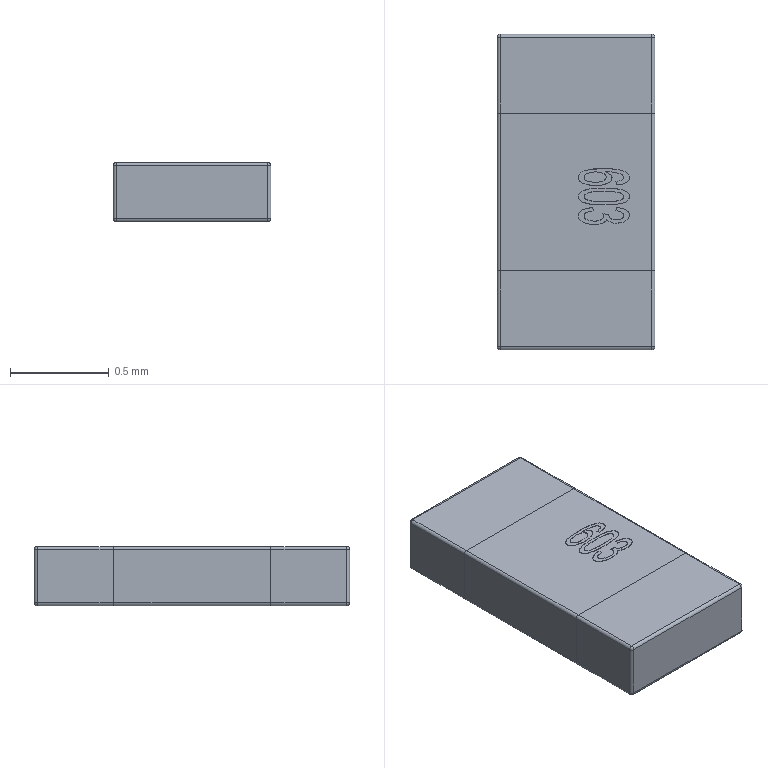Part | STEP file | RJ-USIO-V1_2-220411_132 | 1 solid | 90 faces | box 0.8 x 1.6 x 0.302 mm | volume 0.3835 mm3 | cylinder 31 | other 27 | plane 24 | sphere 8 | commonest cylinder face diameters 0.03 x20 0.038 x1 0.041 x1 0.048 x1 0.053 x1 0.068 x1